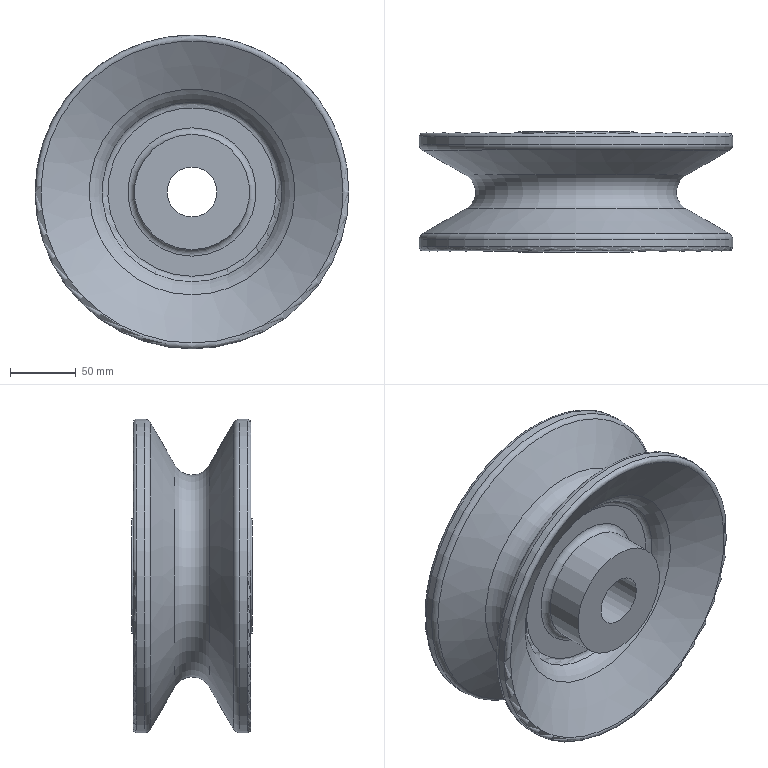Part | NX | features DATUM_CSYS 2, SKETCH 1, SWP104 1 | 1 solid | 24 faces | box 239.492 x 92 x 239.492 mm | volume 1529251 mm3 | torus 11 | cylinder 5 | plane 4 | cone 4 | commonest cylinder face diameters 88 x2 239.492 x2 38 x1
STEP:
#1=CARTESIAN_POINT('',(0.,-46.,-44.));
#2=VERTEX_POINT('',#1);
#3=CARTESIAN_POINT('',(0.,-46.,0.));
#4=DIRECTION('',(0.,-1.,0.));
#5=DIRECTION('',(0.,0.,-1.));
#6=AXIS2_PLACEMENT_3D('',#3,#4,#5);
#7=CIRCLE('',#6,44.);
#8=EDGE_CURVE('',#2,#2,#7,.T.);
#9=ORIENTED_EDGE('',*,*,#8,.T.);
#10=EDGE_LOOP('',(#9));
#11=FACE_BOUND('',#10,.T.);
#12=CARTESIAN_POINT('',(0.,-46.,-19.));
#13=VERTEX_POINT('',#12);
#14=CARTESIAN_POINT('',(0.,-46.,0.));
#15=DIRECTION('',(0.,-1.,0.));
#16=DIRECTION('',(0.,0.,-1.));
#17=AXIS2_PLACEMENT_3D('',#14,#15,#16);
#18=CIRCLE('',#17,19.);
#19=EDGE_CURVE('',#13,#13,#18,.T.);
#20=ORIENTED_EDGE('',*,*,#19,.F.);
#21=EDGE_LOOP('',(#20));
#22=FACE_BOUND('',#21,.T.);
#23=CARTESIAN_POINT('',(0.,-46.,-19.));
#24=DIRECTION('',(0.,-1.,0.));
#25=DIRECTION('',(0.,0.,-1.));
#26=AXIS2_PLACEMENT_3D('',#23,#24,#25);
#27=PLANE('',#26);
#28=ADVANCED_FACE('',(#11,#22),#27,.T.);
#29=CARTESIAN_POINT('',(0.,-16.,-44.));
#30=VERTEX_POINT('',#29);
#31=CARTESIAN_POINT('',(0.,-16.,0.));
#32=DIRECTION('',(0.,-1.,0.));
#33=DIRECTION('',(0.,0.,-1.));
#34=AXIS2_PLACEMENT_3D('',#31,#32,#33);
#35=CIRCLE('',#34,44.);
#36=EDGE_CURVE('',#30,#30,#35,.T.);
#37=ORIENTED_EDGE('',*,*,#36,.T.);
#38=EDGE_LOOP('',(#37));
#39=FACE_BOUND('',#38,.T.);
#40=ORIENTED_EDGE('',*,*,#8,.F.);
#41=EDGE_LOOP('',(#40));
#42=FACE_BOUND('',#41,.T.);
#43=CARTESIAN_POINT('',(0.,0.,0.));
#44=DIRECTION('',(0.,-1.,0.));
#45=DIRECTION('',(0.,0.,-1.));
#46=AXIS2_PLACEMENT_3D('',#43,#44,#45);
#47=CYLINDRICAL_SURFACE('',#46,44.);
#48=ADVANCED_FACE('',(#39,#42),#47,.T.);
#49=CARTESIAN_POINT('',(0.,-11.,-49.));
#50=VERTEX_POINT('',#49);
#51=CARTESIAN_POINT('',(0.,-11.,0.));
#52=DIRECTION('',(0.,-1.,0.));
#53=DIRECTION('',(0.,0.,-1.));
#54=AXIS2_PLACEMENT_3D('',#51,#52,#53);
#55=CIRCLE('',#54,49.);
#56=EDGE_CURVE('',#50,#50,#55,.T.);
#57=ORIENTED_EDGE('',*,*,#56,.T.);
#58=EDGE_LOOP('',(#57));
#59=FACE_BOUND('',#58,.T.);
#60=ORIENTED_EDGE('',*,*,#36,.F.);
#61=EDGE_LOOP('',(#60));
#62=FACE_BOUND('',#61,.T.);
#63=CARTESIAN_POINT('',(0.,-16.,0.));
#64=DIRECTION('',(0.,-1.,0.));
#65=DIRECTION('',(0.,0.,-1.));
#66=AXIS2_PLACEMENT_3D('',#63,#64,#65);
#67=TOROIDAL_SURFACE('',#66,49.,5.);
#68=ADVANCED_FACE('',(#59,#62),#67,.F.);
#69=CARTESIAN_POINT('',(0.,-11.,-64.287));
#70=VERTEX_POINT('',#69);
#71=CARTESIAN_POINT('',(0.,-11.,0.));
#72=DIRECTION('',(0.,-1.,0.));
#73=DIRECTION('',(0.,0.,-1.));
#74=AXIS2_PLACEMENT_3D('',#71,#72,#73);
#75=CIRCLE('',#74,64.287);
#76=EDGE_CURVE('',#70,#70,#75,.T.);
#77=ORIENTED_EDGE('',*,*,#76,.T.);
#78=EDGE_LOOP('',(#77));
#79=FACE_BOUND('',#78,.T.);
#80=ORIENTED_EDGE('',*,*,#56,.F.);
#81=EDGE_LOOP('',(#80));
#82=FACE_BOUND('',#81,.T.);
#83=CARTESIAN_POINT('',(0.,-11.,-49.));
#84=DIRECTION('',(0.,-1.,0.));
#85=DIRECTION('',(0.,0.,-1.));
#86=AXIS2_PLACEMENT_3D('',#83,#84,#85);
#87=PLANE('',#86);
#88=ADVANCED_FACE('',(#79,#82),#87,.T.);
#89=CARTESIAN_POINT('',(0.,-13.5,-68.617));
#90=VERTEX_POINT('',#89);
#91=CARTESIAN_POINT('',(0.,-13.5,0.));
#92=DIRECTION('',(0.,-1.,0.));
#93=DIRECTION('',(0.,0.,-1.));
#94=AXIS2_PLACEMENT_3D('',#91,#92,#93);
#95=CIRCLE('',#94,68.617);
#96=EDGE_CURVE('',#90,#90,#95,.T.);
#97=ORIENTED_EDGE('',*,*,#96,.T.);
#98=EDGE_LOOP('',(#97));
#99=FACE_BOUND('',#98,.T.);
#100=ORIENTED_EDGE('',*,*,#76,.F.);
#101=EDGE_LOOP('',(#100));
#102=FACE_BOUND('',#101,.T.);
#103=CARTESIAN_POINT('',(0.,-16.,0.));
#104=DIRECTION('',(0.,-1.,0.));
#105=DIRECTION('',(0.,0.,-1.));
#106=AXIS2_PLACEMENT_3D('',#103,#104,#105);
#107=TOROIDAL_SURFACE('',#106,64.287,5.);
#108=ADVANCED_FACE('',(#99,#102),#107,.F.);
#109=CARTESIAN_POINT('',(0.,-23.383,-78.5));
#110=VERTEX_POINT('',#109);
#111=CARTESIAN_POINT('',(0.,-23.383,0.));
#112=DIRECTION('',(0.,-1.,0.));
#113=DIRECTION('',(0.,0.,-1.));
#114=AXIS2_PLACEMENT_3D('',#111,#112,#113);
#115=CIRCLE('',#114,78.5);
#116=EDGE_CURVE('',#110,#110,#115,.T.);
#117=ORIENTED_EDGE('',*,*,#116,.T.);
#118=EDGE_LOOP('',(#117));
#119=FACE_BOUND('',#118,.T.);
#120=ORIENTED_EDGE('',*,*,#96,.F.);
#121=EDGE_LOOP('',(#120));
#122=FACE_BOUND('',#121,.T.);
#123=CARTESIAN_POINT('',(0.,0.,0.));
#124=DIRECTION('',(0.,-1.,0.));
#125=DIRECTION('',(0.,0.,-1.));
#126=AXIS2_PLACEMENT_3D('',#123,#124,#125);
#127=TOROIDAL_SURFACE('',#126,92.,27.);
#128=ADVANCED_FACE('',(#119,#122),#127,.T.);
#129=CARTESIAN_POINT('',(0.,-44.598,-115.246));
#130=VERTEX_POINT('',#129);
#131=CARTESIAN_POINT('',(0.,-44.598,0.));
#132=DIRECTION('',(0.,-1.,0.));
#133=DIRECTION('',(0.,0.,-1.));
#134=AXIS2_PLACEMENT_3D('',#131,#132,#133);
#135=CIRCLE('',#134,115.246);
#136=EDGE_CURVE('',#130,#130,#135,.T.);
#137=ORIENTED_EDGE('',*,*,#136,.T.);
#138=EDGE_LOOP('',(#137));
#139=FACE_BOUND('',#138,.T.);
#140=ORIENTED_EDGE('',*,*,#116,.F.);
#141=EDGE_LOOP('',(#140));
#142=FACE_BOUND('',#141,.T.);
#143=CARTESIAN_POINT('',(0.,-23.383,0.));
#144=DIRECTION('',(0.,-1.,0.));
#145=DIRECTION('',(0.,0.,-1.));
#146=AXIS2_PLACEMENT_3D('',#143,#144,#145);
#147=CONICAL_SURFACE('',#146,78.5,1.047);
#148=ADVANCED_FACE('',(#139,#142),#147,.F.);
#149=CARTESIAN_POINT('',(0.,-42.,-119.746));
#150=VERTEX_POINT('',#149);
#151=CARTESIAN_POINT('',(0.,-42.,0.));
#152=DIRECTION('',(0.,-1.,0.));
#153=DIRECTION('',(0.,0.,-1.));
#154=AXIS2_PLACEMENT_3D('',#151,#152,#153);
#155=CIRCLE('',#154,119.746);
#156=EDGE_CURVE('',#150,#150,#155,.T.);
#157=ORIENTED_EDGE('',*,*,#156,.T.);
#158=EDGE_LOOP('',(#157));
#159=FACE_BOUND('',#158,.T.);
#160=ORIENTED_EDGE('',*,*,#136,.F.);
#161=EDGE_LOOP('',(#160));
#162=FACE_BOUND('',#161,.T.);
#163=CARTESIAN_POINT('',(0.,-42.,0.));
#164=DIRECTION('',(0.,-1.,0.));
#165=DIRECTION('',(0.,0.,-1.));
#166=AXIS2_PLACEMENT_3D('',#163,#164,#165);
#167=TOROIDAL_SURFACE('',#166,116.746,3.);
#168=ADVANCED_FACE('',(#159,#162),#167,.T.);
#169=CARTESIAN_POINT('',(0.,-36.226,-119.746));
#170=VERTEX_POINT('',#169);
#171=CARTESIAN_POINT('',(0.,-36.226,0.));
#172=DIRECTION('',(0.,-1.,0.));
#173=DIRECTION('',(0.,0.,-1.));
#174=AXIS2_PLACEMENT_3D('',#171,#172,#173);
#175=CIRCLE('',#174,119.746);
#176=EDGE_CURVE('',#170,#170,#175,.T.);
#177=ORIENTED_EDGE('',*,*,#176,.T.);
#178=EDGE_LOOP('',(#177));
#179=FACE_BOUND('',#178,.T.);
#180=ORIENTED_EDGE('',*,*,#156,.F.);
#181=EDGE_LOOP('',(#180));
#182=FACE_BOUND('',#181,.T.);
#183=CARTESIAN_POINT('',(0.,0.,0.));
#184=DIRECTION('',(0.,-1.,0.));
#185=DIRECTION('',(0.,0.,-1.));
#186=AXIS2_PLACEMENT_3D('',#183,#184,#185);
#187=CYLINDRICAL_SURFACE('',#186,119.746);
#188=ADVANCED_FACE('',(#179,#182),#187,.T.);
#189=CARTESIAN_POINT('',(0.,-31.896,-117.246));
#190=VERTEX_POINT('',#189);
#191=CARTESIAN_POINT('',(0.,-31.896,0.));
#192=DIRECTION('',(0.,-1.,0.));
#193=DIRECTION('',(0.,0.,-1.));
#194=AXIS2_PLACEMENT_3D('',#191,#192,#193);
#195=CIRCLE('',#194,117.246);
#196=EDGE_CURVE('',#190,#190,#195,.T.);
#197=ORIENTED_EDGE('',*,*,#196,.T.);
#198=EDGE_LOOP('',(#197));
#199=FACE_BOUND('',#198,.T.);
#200=ORIENTED_EDGE('',*,*,#176,.F.);
#201=EDGE_LOOP('',(#200));
#202=FACE_BOUND('',#201,.T.);
#203=CARTESIAN_POINT('',(0.,-36.226,0.));
#204=DIRECTION('',(0.,-1.,0.));
#205=DIRECTION('',(0.,0.,-1.));
#206=AXIS2_PLACEMENT_3D('',#203,#204,#205);
#207=TOROIDAL_SURFACE('',#206,114.746,5.);
#208=ADVANCED_FACE('',(#199,#202),#207,.T.);
#209=CARTESIAN_POINT('',(0.,-12.99,-84.5));
#210=VERTEX_POINT('',#209);
#211=CARTESIAN_POINT('',(0.,-12.99,0.));
#212=DIRECTION('',(0.,-1.,0.));
#213=DIRECTION('',(0.,0.,-1.));
#214=AXIS2_PLACEMENT_3D('',#211,#212,#213);
#215=CIRCLE('',#214,84.5);
#216=EDGE_CURVE('',#210,#210,#215,.T.);
#217=ORIENTED_EDGE('',*,*,#216,.T.);
#218=EDGE_LOOP('',(#217));
#219=FACE_BOUND('',#218,.T.);
#220=ORIENTED_EDGE('',*,*,#196,.F.);
#221=EDGE_LOOP('',(#220));
#222=FACE_BOUND('',#221,.T.);
#223=CARTESIAN_POINT('',(0.,-31.896,0.));
#224=DIRECTION('',(0.,-1.,0.));
#225=DIRECTION('',(0.,0.,-1.));
#226=AXIS2_PLACEMENT_3D('',#223,#224,#225);
#227=CONICAL_SURFACE('',#226,117.246,1.047);
#228=ADVANCED_FACE('',(#219,#222),#227,.T.);
#229=CARTESIAN_POINT('',(0.,12.99,-84.5));
#230=VERTEX_POINT('',#229);
#231=CARTESIAN_POINT('',(0.,12.99,0.));
#232=DIRECTION('',(0.,-1.,0.));
#233=DIRECTION('',(0.,0.,-1.));
#234=AXIS2_PLACEMENT_3D('',#231,#232,#233);
#235=CIRCLE('',#234,84.5);
#236=EDGE_CURVE('',#230,#230,#235,.T.);
#237=ORIENTED_EDGE('',*,*,#236,.T.);
#238=EDGE_LOOP('',(#237));
#239=FACE_BOUND('',#238,.T.);
#240=ORIENTED_EDGE('',*,*,#216,.F.);
#241=EDGE_LOOP('',(#240));
#242=FACE_BOUND('',#241,.T.);
#243=CARTESIAN_POINT('',(0.,0.,0.));
#244=DIRECTION('',(0.,-1.,0.));
#245=DIRECTION('',(0.,0.,-1.));
#246=AXIS2_PLACEMENT_3D('',#243,#244,#245);
#247=TOROIDAL_SURFACE('',#246,92.,15.);
#248=ADVANCED_FACE('',(#239,#242),#247,.F.);
#249=CARTESIAN_POINT('',(0.,31.896,-117.246));
#250=VERTEX_POINT('',#249);
#251=CARTESIAN_POINT('',(0.,31.896,0.));
#252=DIRECTION('',(0.,-1.,0.));
#253=DIRECTION('',(0.,0.,-1.));
#254=AXIS2_PLACEMENT_3D('',#251,#252,#253);
#255=CIRCLE('',#254,117.246);
#256=EDGE_CURVE('',#250,#250,#255,.T.);
#257=ORIENTED_EDGE('',*,*,#256,.T.);
#258=EDGE_LOOP('',(#257));
#259=FACE_BOUND('',#258,.T.);
#260=ORIENTED_EDGE('',*,*,#236,.F.);
#261=EDGE_LOOP('',(#260));
#262=FACE_BOUND('',#261,.T.);
#263=CARTESIAN_POINT('',(0.,12.99,0.));
#264=DIRECTION('',(0.,1.,0.));
#265=DIRECTION('',(0.,0.,1.));
#266=AXIS2_PLACEMENT_3D('',#263,#264,#265);
#267=CONICAL_SURFACE('',#266,84.5,1.047);
#268=ADVANCED_FACE('',(#259,#262),#267,.T.);
#269=CARTESIAN_POINT('',(0.,36.226,-119.746));
#270=VERTEX_POINT('',#269);
#271=CARTESIAN_POINT('',(0.,36.226,0.));
#272=DIRECTION('',(0.,-1.,0.));
#273=DIRECTION('',(0.,0.,-1.));
#274=AXIS2_PLACEMENT_3D('',#271,#272,#273);
#275=CIRCLE('',#274,119.746);
#276=EDGE_CURVE('',#270,#270,#275,.T.);
#277=ORIENTED_EDGE('',*,*,#276,.T.);
#278=EDGE_LOOP('',(#277));
#279=FACE_BOUND('',#278,.T.);
#280=ORIENTED_EDGE('',*,*,#256,.F.);
#281=EDGE_LOOP('',(#280));
#282=FACE_BOUND('',#281,.T.);
#283=CARTESIAN_POINT('',(0.,36.226,0.));
#284=DIRECTION('',(0.,-1.,0.));
#285=DIRECTION('',(0.,0.,-1.));
#286=AXIS2_PLACEMENT_3D('',#283,#284,#285);
#287=TOROIDAL_SURFACE('',#286,114.746,5.);
#288=ADVANCED_FACE('',(#279,#282),#287,.T.);
#289=CARTESIAN_POINT('',(0.,42.,-119.746));
#290=VERTEX_POINT('',#289);
#291=CARTESIAN_POINT('',(0.,42.,0.));
#292=DIRECTION('',(0.,-1.,0.));
#293=DIRECTION('',(0.,0.,-1.));
#294=AXIS2_PLACEMENT_3D('',#291,#292,#293);
#295=CIRCLE('',#294,119.746);
#296=EDGE_CURVE('',#290,#290,#295,.T.);
#297=ORIENTED_EDGE('',*,*,#296,.T.);
#298=EDGE_LOOP('',(#297));
#299=FACE_BOUND('',#298,.T.);
#300=ORIENTED_EDGE('',*,*,#276,.F.);
#301=EDGE_LOOP('',(#300));
#302=FACE_BOUND('',#301,.T.);
#303=CARTESIAN_POINT('',(0.,0.,0.));
#304=DIRECTION('',(0.,-1.,0.));
#305=DIRECTION('',(0.,0.,-1.));
#306=AXIS2_PLACEMENT_3D('',#303,#304,#305);
#307=CYLINDRICAL_SURFACE('',#306,119.746);
#308=ADVANCED_FACE('',(#299,#302),#307,.T.);
#309=CARTESIAN_POINT('',(0.,44.598,-115.246));
#310=VERTEX_POINT('',#309);
#311=CARTESIAN_POINT('',(0.,44.598,0.));
#312=DIRECTION('',(0.,-1.,0.));
#313=DIRECTION('',(0.,0.,-1.));
#314=AXIS2_PLACEMENT_3D('',#311,#312,#313);
#315=CIRCLE('',#314,115.246);
#316=EDGE_CURVE('',#310,#310,#315,.T.);
#317=ORIENTED_EDGE('',*,*,#316,.T.);
#318=EDGE_LOOP('',(#317));
#319=FACE_BOUND('',#318,.T.);
#320=ORIENTED_EDGE('',*,*,#296,.F.);
#321=EDGE_LOOP('',(#320));
#322=FACE_BOUND('',#321,.T.);
#323=CARTESIAN_POINT('',(0.,42.,0.));
#324=DIRECTION('',(0.,-1.,0.));
#325=DIRECTION('',(0.,0.,-1.));
#326=AXIS2_PLACEMENT_3D('',#323,#324,#325);
#327=TOROIDAL_SURFACE('',#326,116.746,3.);
#328=ADVANCED_FACE('',(#319,#322),#327,.T.);
#329=CARTESIAN_POINT('',(0.,23.383,-78.5));
#330=VERTEX_POINT('',#329);
#331=CARTESIAN_POINT('',(0.,23.383,0.));
#332=DIRECTION('',(0.,-1.,0.));
#333=DIRECTION('',(0.,0.,-1.));
#334=AXIS2_PLACEMENT_3D('',#331,#332,#333);
#335=CIRCLE('',#334,78.5);
#336=EDGE_CURVE('',#330,#330,#335,.T.);
#337=ORIENTED_EDGE('',*,*,#336,.T.);
#338=EDGE_LOOP('',(#337));
#339=FACE_BOUND('',#338,.T.);
#340=ORIENTED_EDGE('',*,*,#316,.F.);
#341=EDGE_LOOP('',(#340));
#342=FACE_BOUND('',#341,.T.);
#343=CARTESIAN_POINT('',(0.,44.598,0.));
#344=DIRECTION('',(0.,1.,0.));
#345=DIRECTION('',(0.,0.,1.));
#346=AXIS2_PLACEMENT_3D('',#343,#344,#345);
#347=CONICAL_SURFACE('',#346,115.246,1.047);
#348=ADVANCED_FACE('',(#339,#342),#347,.F.);
#349=CARTESIAN_POINT('',(0.,13.5,-68.617));
#350=VERTEX_POINT('',#349);
#351=CARTESIAN_POINT('',(0.,13.5,0.));
#352=DIRECTION('',(0.,-1.,0.));
#353=DIRECTION('',(0.,0.,-1.));
#354=AXIS2_PLACEMENT_3D('',#351,#352,#353);
#355=CIRCLE('',#354,68.617);
#356=EDGE_CURVE('',#350,#350,#355,.T.);
#357=ORIENTED_EDGE('',*,*,#356,.T.);
#358=EDGE_LOOP('',(#357));
#359=FACE_BOUND('',#358,.T.);
#360=ORIENTED_EDGE('',*,*,#336,.F.);
#361=EDGE_LOOP('',(#360));
#362=FACE_BOUND('',#361,.T.);
#363=CARTESIAN_POINT('',(0.,0.,0.));
#364=DIRECTION('',(0.,-1.,0.));
#365=DIRECTION('',(0.,0.,-1.));
#366=AXIS2_PLACEMENT_3D('',#363,#364,#365);
#367=TOROIDAL_SURFACE('',#366,92.,27.);
#368=ADVANCED_FACE('',(#359,#362),#367,.T.);
#369=CARTESIAN_POINT('',(0.,11.,-64.287));
#370=VERTEX_POINT('',#369);
#371=CARTESIAN_POINT('',(0.,11.,0.));
#372=DIRECTION('',(0.,-1.,0.));
#373=DIRECTION('',(0.,0.,-1.));
#374=AXIS2_PLACEMENT_3D('',#371,#372,#373);
#375=CIRCLE('',#374,64.287);
#376=EDGE_CURVE('',#370,#370,#375,.T.);
#377=ORIENTED_EDGE('',*,*,#376,.T.);
#378=EDGE_LOOP('',(#377));
#379=FACE_BOUND('',#378,.T.);
#380=ORIENTED_EDGE('',*,*,#356,.F.);
#381=EDGE_LOOP('',(#380));
#382=FACE_BOUND('',#381,.T.);
#383=CARTESIAN_POINT('',(0.,16.,0.));
#384=DIRECTION('',(0.,-1.,0.));
#385=DIRECTION('',(0.,0.,-1.));
#386=AXIS2_PLACEMENT_3D('',#383,#384,#385);
#387=TOROIDAL_SURFACE('',#386,64.287,5.);
#388=ADVANCED_FACE('',(#379,#382),#387,.F.);
#389=CARTESIAN_POINT('',(0.,11.,-49.));
#390=VERTEX_POINT('',#389);
#391=CARTESIAN_POINT('',(0.,11.,0.));
#392=DIRECTION('',(0.,-1.,0.));
#393=DIRECTION('',(0.,0.,-1.));
#394=AXIS2_PLACEMENT_3D('',#391,#392,#393);
#395=CIRCLE('',#394,49.);
#396=EDGE_CURVE('',#390,#390,#395,.T.);
#397=ORIENTED_EDGE('',*,*,#396,.T.);
#398=EDGE_LOOP('',(#397));
#399=FACE_BOUND('',#398,.T.);
#400=ORIENTED_EDGE('',*,*,#376,.F.);
#401=EDGE_LOOP('',(#400));
#402=FACE_BOUND('',#401,.T.);
#403=CARTESIAN_POINT('',(0.,11.,-64.287));
#404=DIRECTION('',(0.,1.,0.));
#405=DIRECTION('',(0.,0.,1.));
#406=AXIS2_PLACEMENT_3D('',#403,#404,#405);
#407=PLANE('',#406);
#408=ADVANCED_FACE('',(#399,#402),#407,.T.);
#409=CARTESIAN_POINT('',(0.,16.,-44.));
#410=VERTEX_POINT('',#409);
#411=CARTESIAN_POINT('',(0.,16.,0.));
#412=DIRECTION('',(0.,-1.,0.));
#413=DIRECTION('',(0.,0.,-1.));
#414=AXIS2_PLACEMENT_3D('',#411,#412,#413);
#415=CIRCLE('',#414,44.);
#416=EDGE_CURVE('',#410,#410,#415,.T.);
#417=ORIENTED_EDGE('',*,*,#416,.T.);
#418=EDGE_LOOP('',(#417));
#419=FACE_BOUND('',#418,.T.);
#420=ORIENTED_EDGE('',*,*,#396,.F.);
#421=EDGE_LOOP('',(#420));
#422=FACE_BOUND('',#421,.T.);
#423=CARTESIAN_POINT('',(0.,16.,0.));
#424=DIRECTION('',(0.,-1.,0.));
#425=DIRECTION('',(0.,0.,-1.));
#426=AXIS2_PLACEMENT_3D('',#423,#424,#425);
#427=TOROIDAL_SURFACE('',#426,49.,5.);
#428=ADVANCED_FACE('',(#419,#422),#427,.F.);
#429=CARTESIAN_POINT('',(0.,46.,-44.));
#430=VERTEX_POINT('',#429);
#431=CARTESIAN_POINT('',(0.,46.,0.));
#432=DIRECTION('',(0.,-1.,0.));
#433=DIRECTION('',(0.,0.,-1.));
#434=AXIS2_PLACEMENT_3D('',#431,#432,#433);
#435=CIRCLE('',#434,44.);
#436=EDGE_CURVE('',#430,#430,#435,.T.);
#437=ORIENTED_EDGE('',*,*,#436,.T.);
#438=EDGE_LOOP('',(#437));
#439=FACE_BOUND('',#438,.T.);
#440=ORIENTED_EDGE('',*,*,#416,.F.);
#441=EDGE_LOOP('',(#440));
#442=FACE_BOUND('',#441,.T.);
#443=CARTESIAN_POINT('',(0.,0.,0.));
#444=DIRECTION('',(0.,-1.,0.));
#445=DIRECTION('',(0.,0.,-1.));
#446=AXIS2_PLACEMENT_3D('',#443,#444,#445);
#447=CYLINDRICAL_SURFACE('',#446,44.);
#448=ADVANCED_FACE('',(#439,#442),#447,.T.);
#449=CARTESIAN_POINT('',(0.,46.,-19.));
#450=VERTEX_POINT('',#449);
#451=CARTESIAN_POINT('',(0.,46.,0.));
#452=DIRECTION('',(0.,-1.,0.));
#453=DIRECTION('',(0.,0.,-1.));
#454=AXIS2_PLACEMENT_3D('',#451,#452,#453);
#455=CIRCLE('',#454,19.);
#456=EDGE_CURVE('',#450,#450,#455,.T.);
#457=ORIENTED_EDGE('',*,*,#456,.T.);
#458=EDGE_LOOP('',(#457));
#459=FACE_BOUND('',#458,.T.);
#460=ORIENTED_EDGE('',*,*,#436,.F.);
#461=EDGE_LOOP('',(#460));
#462=FACE_BOUND('',#461,.T.);
#463=CARTESIAN_POINT('',(0.,46.,-44.));
#464=DIRECTION('',(0.,1.,0.));
#465=DIRECTION('',(0.,0.,1.));
#466=AXIS2_PLACEMENT_3D('',#463,#464,#465);
#467=PLANE('',#466);
#468=ADVANCED_FACE('',(#459,#462),#467,.T.);
#469=ORIENTED_EDGE('',*,*,#19,.T.);
#470=EDGE_LOOP('',(#469));
#471=FACE_BOUND('',#470,.T.);
#472=ORIENTED_EDGE('',*,*,#456,.F.);
#473=EDGE_LOOP('',(#472));
#474=FACE_BOUND('',#473,.T.);
#475=CARTESIAN_POINT('',(0.,0.,0.));
#476=DIRECTION('',(0.,-1.,0.));
#477=DIRECTION('',(0.,0.,-1.));
#478=AXIS2_PLACEMENT_3D('',#475,#476,#477);
#479=CYLINDRICAL_SURFACE('',#478,19.);
#480=ADVANCED_FACE('',(#471,#474),#479,.F.);
#481=CLOSED_SHELL('',(#28,#48,#68,#88,#108,#128,#148,#168,#188,#208,#228,#248,#268,#288,#308,#328,#348,#368,#388,#408,#428,#448,#468,#480));
#482=MANIFOLD_SOLID_BREP('',#481);
#483=(LENGTH_UNIT()NAMED_UNIT(*)SI_UNIT(.MILLI.,.METRE.));
#484=UNCERTAINTY_MEASURE_WITH_UNIT(LENGTH_MEASURE(0.00001),#483,'','');
#485=(NAMED_UNIT(*)PLANE_ANGLE_UNIT()SI_UNIT($,.RADIAN.));
#486=(NAMED_UNIT(*)SI_UNIT($,.STERADIAN.)SOLID_ANGLE_UNIT());
#487=(GEOMETRIC_REPRESENTATION_CONTEXT(3)GLOBAL_UNCERTAINTY_ASSIGNED_CONTEXT((#484))GLOBAL_UNIT_ASSIGNED_CONTEXT((#483,#485,#486))REPRESENTATION_CONTEXT('',''));
#488=ADVANCED_BREP_SHAPE_REPRESENTATION('',(#482),#487);